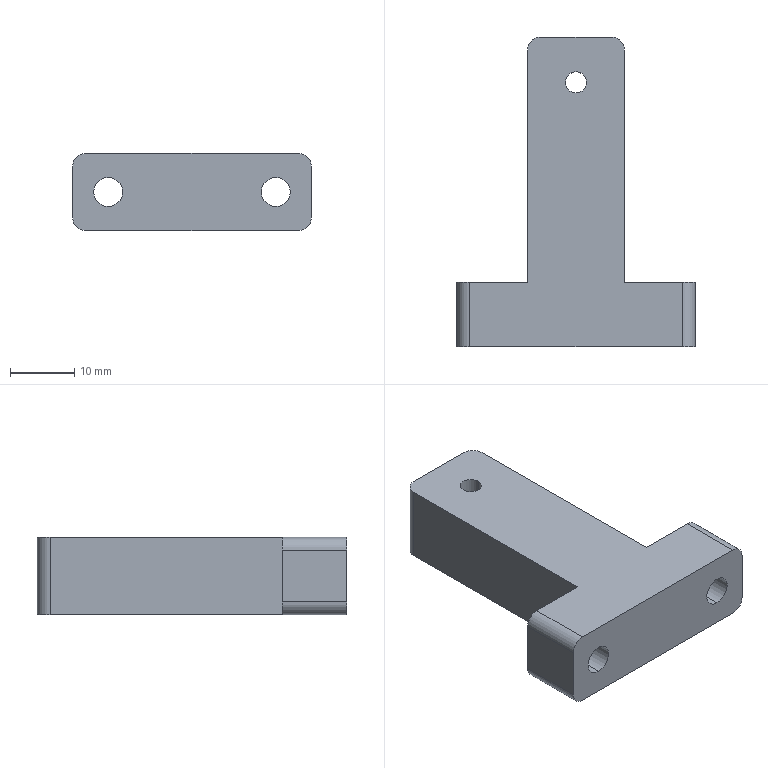Part | NX | features BREP 1 | 1 solid | 28 faces | box 37 x 48 x 12 mm | volume 10327 mm3 | cylinder 16 | plane 12 | commonest cylinder face diameters 4 x6 4.5 x4 9 x4 3.3 x2
STEP:
#1=CARTESIAN_POINT('',(7.5,46.,6.));
#2=VERTEX_POINT('',#1);
#3=CARTESIAN_POINT('',(5.5,48.,6.));
#4=VERTEX_POINT('',#3);
#5=CARTESIAN_POINT('',(5.5,46.,6.));
#6=DIRECTION('',(0.,0.,1.));
#7=DIRECTION('',(-1.,0.,0.));
#8=AXIS2_PLACEMENT_3D('',#5,#6,#7);
#9=CIRCLE('',#8,2.);
#10=EDGE_CURVE('',#2,#4,#9,.T.);
#11=ORIENTED_EDGE('',*,*,#10,.F.);
#12=CARTESIAN_POINT('',(7.5,46.,-6.));
#13=VERTEX_POINT('',#12);
#14=CARTESIAN_POINT('',(7.5,46.,6.));
#15=DIRECTION('',(0.,0.,1.));
#16=VECTOR('',#15,1000.);
#17=LINE('',#14,#16);
#18=EDGE_CURVE('',#13,#2,#17,.T.);
#19=ORIENTED_EDGE('',*,*,#18,.F.);
#20=CARTESIAN_POINT('',(5.5,48.,-6.));
#21=VERTEX_POINT('',#20);
#22=CARTESIAN_POINT('',(5.5,46.,-6.));
#23=DIRECTION('',(0.,0.,-1.));
#24=DIRECTION('',(-1.,0.,0.));
#25=AXIS2_PLACEMENT_3D('',#22,#23,#24);
#26=CIRCLE('',#25,2.);
#27=EDGE_CURVE('',#21,#13,#26,.T.);
#28=ORIENTED_EDGE('',*,*,#27,.F.);
#29=CARTESIAN_POINT('',(5.5,48.,6.));
#30=DIRECTION('',(0.,0.,-1.));
#31=VECTOR('',#30,1000.);
#32=LINE('',#29,#31);
#33=EDGE_CURVE('',#4,#21,#32,.T.);
#34=ORIENTED_EDGE('',*,*,#33,.F.);
#35=EDGE_LOOP('',(#11,#19,#28,#34));
#36=FACE_BOUND('',#35,.T.);
#37=CARTESIAN_POINT('',(5.5,46.,6.));
#38=DIRECTION('',(0.,0.,-1.));
#39=DIRECTION('',(-1.,0.,0.));
#40=AXIS2_PLACEMENT_3D('',#37,#38,#39);
#41=CYLINDRICAL_SURFACE('',#40,2.);
#42=ADVANCED_FACE('',(#36),#41,.T.);
#43=CARTESIAN_POINT('',(-5.5,48.,6.));
#44=VERTEX_POINT('',#43);
#45=CARTESIAN_POINT('',(-7.5,46.,6.));
#46=VERTEX_POINT('',#45);
#47=CARTESIAN_POINT('',(-5.5,46.,6.));
#48=DIRECTION('',(0.,0.,1.));
#49=DIRECTION('',(-1.,0.,0.));
#50=AXIS2_PLACEMENT_3D('',#47,#48,#49);
#51=CIRCLE('',#50,2.);
#52=EDGE_CURVE('',#44,#46,#51,.T.);
#53=ORIENTED_EDGE('',*,*,#52,.F.);
#54=CARTESIAN_POINT('',(-5.5,48.,-6.));
#55=VERTEX_POINT('',#54);
#56=CARTESIAN_POINT('',(-5.5,48.,6.));
#57=DIRECTION('',(0.,0.,1.));
#58=VECTOR('',#57,1000.);
#59=LINE('',#56,#58);
#60=EDGE_CURVE('',#55,#44,#59,.T.);
#61=ORIENTED_EDGE('',*,*,#60,.F.);
#62=CARTESIAN_POINT('',(-7.5,46.,-6.));
#63=VERTEX_POINT('',#62);
#64=CARTESIAN_POINT('',(-5.5,46.,-6.));
#65=DIRECTION('',(0.,0.,-1.));
#66=DIRECTION('',(-1.,0.,0.));
#67=AXIS2_PLACEMENT_3D('',#64,#65,#66);
#68=CIRCLE('',#67,2.);
#69=EDGE_CURVE('',#63,#55,#68,.T.);
#70=ORIENTED_EDGE('',*,*,#69,.F.);
#71=CARTESIAN_POINT('',(-7.5,46.,6.));
#72=DIRECTION('',(0.,0.,-1.));
#73=VECTOR('',#72,1000.);
#74=LINE('',#71,#73);
#75=EDGE_CURVE('',#46,#63,#74,.T.);
#76=ORIENTED_EDGE('',*,*,#75,.F.);
#77=EDGE_LOOP('',(#53,#61,#70,#76));
#78=FACE_BOUND('',#77,.T.);
#79=CARTESIAN_POINT('',(-5.5,46.,6.));
#80=DIRECTION('',(0.,0.,-1.));
#81=DIRECTION('',(-1.,0.,0.));
#82=AXIS2_PLACEMENT_3D('',#79,#80,#81);
#83=CYLINDRICAL_SURFACE('',#82,2.);
#84=ADVANCED_FACE('',(#78),#83,.T.);
#85=CARTESIAN_POINT('',(16.5,0.,-6.));
#86=VERTEX_POINT('',#85);
#87=CARTESIAN_POINT('',(18.5,0.,-4.));
#88=VERTEX_POINT('',#87);
#89=CARTESIAN_POINT('',(16.5,0.,-4.));
#90=DIRECTION('',(0.,-1.,0.));
#91=DIRECTION('',(0.,0.,1.));
#92=AXIS2_PLACEMENT_3D('',#89,#90,#91);
#93=CIRCLE('',#92,2.);
#94=EDGE_CURVE('',#86,#88,#93,.T.);
#95=ORIENTED_EDGE('',*,*,#94,.F.);
#96=CARTESIAN_POINT('',(16.5,10.,-6.));
#97=VERTEX_POINT('',#96);
#98=CARTESIAN_POINT('',(16.5,0.,-6.));
#99=DIRECTION('',(0.,-1.,0.));
#100=VECTOR('',#99,1000.);
#101=LINE('',#98,#100);
#102=EDGE_CURVE('',#97,#86,#101,.T.);
#103=ORIENTED_EDGE('',*,*,#102,.F.);
#104=CARTESIAN_POINT('',(18.5,10.,-4.));
#105=VERTEX_POINT('',#104);
#106=CARTESIAN_POINT('',(16.5,10.,-4.));
#107=DIRECTION('',(0.,1.,0.));
#108=DIRECTION('',(1.,0.,0.));
#109=AXIS2_PLACEMENT_3D('',#106,#107,#108);
#110=CIRCLE('',#109,2.);
#111=EDGE_CURVE('',#105,#97,#110,.T.);
#112=ORIENTED_EDGE('',*,*,#111,.F.);
#113=CARTESIAN_POINT('',(18.5,10.,-4.));
#114=DIRECTION('',(0.,1.,0.));
#115=VECTOR('',#114,1000.);
#116=LINE('',#113,#115);
#117=EDGE_CURVE('',#88,#105,#116,.T.);
#118=ORIENTED_EDGE('',*,*,#117,.F.);
#119=EDGE_LOOP('',(#95,#103,#112,#118));
#120=FACE_BOUND('',#119,.T.);
#121=CARTESIAN_POINT('',(16.5,10.,-4.));
#122=DIRECTION('',(0.,-1.,0.));
#123=DIRECTION('',(1.,0.,0.));
#124=AXIS2_PLACEMENT_3D('',#121,#122,#123);
#125=CYLINDRICAL_SURFACE('',#124,2.);
#126=ADVANCED_FACE('',(#120),#125,.T.);
#127=CARTESIAN_POINT('',(18.5,0.,4.));
#128=VERTEX_POINT('',#127);
#129=CARTESIAN_POINT('',(16.5,0.,6.));
#130=VERTEX_POINT('',#129);
#131=CARTESIAN_POINT('',(16.5,0.,4.));
#132=DIRECTION('',(0.,-1.,0.));
#133=DIRECTION('',(0.,0.,1.));
#134=AXIS2_PLACEMENT_3D('',#131,#132,#133);
#135=CIRCLE('',#134,2.);
#136=EDGE_CURVE('',#128,#130,#135,.T.);
#137=ORIENTED_EDGE('',*,*,#136,.F.);
#138=CARTESIAN_POINT('',(18.5,10.,4.));
#139=VERTEX_POINT('',#138);
#140=CARTESIAN_POINT('',(18.5,10.,4.));
#141=DIRECTION('',(0.,-1.,0.));
#142=VECTOR('',#141,1000.);
#143=LINE('',#140,#142);
#144=EDGE_CURVE('',#139,#128,#143,.T.);
#145=ORIENTED_EDGE('',*,*,#144,.F.);
#146=CARTESIAN_POINT('',(16.5,10.,6.));
#147=VERTEX_POINT('',#146);
#148=CARTESIAN_POINT('',(16.5,10.,4.));
#149=DIRECTION('',(0.,1.,0.));
#150=DIRECTION('',(1.,0.,0.));
#151=AXIS2_PLACEMENT_3D('',#148,#149,#150);
#152=CIRCLE('',#151,2.);
#153=EDGE_CURVE('',#147,#139,#152,.T.);
#154=ORIENTED_EDGE('',*,*,#153,.F.);
#155=CARTESIAN_POINT('',(16.5,0.,6.));
#156=DIRECTION('',(0.,1.,0.));
#157=VECTOR('',#156,1000.);
#158=LINE('',#155,#157);
#159=EDGE_CURVE('',#130,#147,#158,.T.);
#160=ORIENTED_EDGE('',*,*,#159,.F.);
#161=EDGE_LOOP('',(#137,#145,#154,#160));
#162=FACE_BOUND('',#161,.T.);
#163=CARTESIAN_POINT('',(16.5,0.,4.));
#164=DIRECTION('',(0.,1.,0.));
#165=DIRECTION('',(-1.,0.,0.));
#166=AXIS2_PLACEMENT_3D('',#163,#164,#165);
#167=CYLINDRICAL_SURFACE('',#166,2.);
#168=ADVANCED_FACE('',(#162),#167,.T.);
#169=CARTESIAN_POINT('',(-16.5,10.,-6.));
#170=VERTEX_POINT('',#169);
#171=CARTESIAN_POINT('',(-18.5,10.,-4.));
#172=VERTEX_POINT('',#171);
#173=CARTESIAN_POINT('',(-16.5,10.,-4.));
#174=DIRECTION('',(0.,1.,0.));
#175=DIRECTION('',(1.,0.,0.));
#176=AXIS2_PLACEMENT_3D('',#173,#174,#175);
#177=CIRCLE('',#176,2.);
#178=EDGE_CURVE('',#170,#172,#177,.T.);
#179=ORIENTED_EDGE('',*,*,#178,.F.);
#180=CARTESIAN_POINT('',(-16.5,0.,-6.));
#181=VERTEX_POINT('',#180);
#182=CARTESIAN_POINT('',(-16.5,10.,-6.));
#183=DIRECTION('',(0.,1.,0.));
#184=VECTOR('',#183,1000.);
#185=LINE('',#182,#184);
#186=EDGE_CURVE('',#181,#170,#185,.T.);
#187=ORIENTED_EDGE('',*,*,#186,.F.);
#188=CARTESIAN_POINT('',(-18.5,0.,-4.));
#189=VERTEX_POINT('',#188);
#190=CARTESIAN_POINT('',(-16.5,0.,-4.));
#191=DIRECTION('',(0.,-1.,0.));
#192=DIRECTION('',(0.,0.,1.));
#193=AXIS2_PLACEMENT_3D('',#190,#191,#192);
#194=CIRCLE('',#193,2.);
#195=EDGE_CURVE('',#189,#181,#194,.T.);
#196=ORIENTED_EDGE('',*,*,#195,.F.);
#197=CARTESIAN_POINT('',(-18.5,0.,-4.));
#198=DIRECTION('',(0.,-1.,0.));
#199=VECTOR('',#198,1000.);
#200=LINE('',#197,#199);
#201=EDGE_CURVE('',#172,#189,#200,.T.);
#202=ORIENTED_EDGE('',*,*,#201,.F.);
#203=EDGE_LOOP('',(#179,#187,#196,#202));
#204=FACE_BOUND('',#203,.T.);
#205=CARTESIAN_POINT('',(-16.5,10.,-4.));
#206=DIRECTION('',(0.,1.,0.));
#207=DIRECTION('',(-1.,0.,0.));
#208=AXIS2_PLACEMENT_3D('',#205,#206,#207);
#209=CYLINDRICAL_SURFACE('',#208,2.);
#210=ADVANCED_FACE('',(#204),#209,.T.);
#211=CARTESIAN_POINT('',(-18.5,10.,4.));
#212=VERTEX_POINT('',#211);
#213=CARTESIAN_POINT('',(-16.5,10.,6.));
#214=VERTEX_POINT('',#213);
#215=CARTESIAN_POINT('',(-16.5,10.,4.));
#216=DIRECTION('',(0.,1.,0.));
#217=DIRECTION('',(1.,0.,0.));
#218=AXIS2_PLACEMENT_3D('',#215,#216,#217);
#219=CIRCLE('',#218,2.);
#220=EDGE_CURVE('',#212,#214,#219,.T.);
#221=ORIENTED_EDGE('',*,*,#220,.F.);
#222=CARTESIAN_POINT('',(-18.5,0.,4.));
#223=VERTEX_POINT('',#222);
#224=CARTESIAN_POINT('',(-18.5,10.,4.));
#225=DIRECTION('',(0.,1.,0.));
#226=VECTOR('',#225,1000.);
#227=LINE('',#224,#226);
#228=EDGE_CURVE('',#223,#212,#227,.T.);
#229=ORIENTED_EDGE('',*,*,#228,.F.);
#230=CARTESIAN_POINT('',(-16.5,0.,6.));
#231=VERTEX_POINT('',#230);
#232=CARTESIAN_POINT('',(-16.5,0.,4.));
#233=DIRECTION('',(0.,-1.,0.));
#234=DIRECTION('',(0.,0.,1.));
#235=AXIS2_PLACEMENT_3D('',#232,#233,#234);
#236=CIRCLE('',#235,2.);
#237=EDGE_CURVE('',#231,#223,#236,.T.);
#238=ORIENTED_EDGE('',*,*,#237,.F.);
#239=CARTESIAN_POINT('',(-16.5,0.,6.));
#240=DIRECTION('',(0.,-1.,0.));
#241=VECTOR('',#240,1000.);
#242=LINE('',#239,#241);
#243=EDGE_CURVE('',#214,#231,#242,.T.);
#244=ORIENTED_EDGE('',*,*,#243,.F.);
#245=EDGE_LOOP('',(#221,#229,#238,#244));
#246=FACE_BOUND('',#245,.T.);
#247=CARTESIAN_POINT('',(-16.5,0.,4.));
#248=DIRECTION('',(0.,-1.,0.));
#249=DIRECTION('',(1.,0.,0.));
#250=AXIS2_PLACEMENT_3D('',#247,#248,#249);
#251=CYLINDRICAL_SURFACE('',#250,2.);
#252=ADVANCED_FACE('',(#246),#251,.T.);
#253=CARTESIAN_POINT('',(-1.65,41.,6.));
#254=VERTEX_POINT('',#253);
#255=CARTESIAN_POINT('',(-1.65,41.,-6.));
#256=VERTEX_POINT('',#255);
#257=CARTESIAN_POINT('',(-1.65,41.,6.));
#258=DIRECTION('',(0.,0.,1.));
#259=VECTOR('',#258,1000.);
#260=LINE('',#257,#259);
#261=EDGE_CURVE('',#254,#256,#260,.F.);
#262=ORIENTED_EDGE('',*,*,#261,.T.);
#263=CARTESIAN_POINT('',(1.65,41.,-6.));
#264=VERTEX_POINT('',#263);
#265=CARTESIAN_POINT('',(0.,41.,-6.));
#266=DIRECTION('',(0.,0.,-1.));
#267=DIRECTION('',(-1.,0.,0.));
#268=AXIS2_PLACEMENT_3D('',#265,#266,#267);
#269=CIRCLE('',#268,1.65);
#270=EDGE_CURVE('',#256,#264,#269,.T.);
#271=ORIENTED_EDGE('',*,*,#270,.T.);
#272=CARTESIAN_POINT('',(1.65,41.,6.));
#273=VERTEX_POINT('',#272);
#274=CARTESIAN_POINT('',(1.65,41.,6.));
#275=DIRECTION('',(0.,0.,1.));
#276=VECTOR('',#275,1000.);
#277=LINE('',#274,#276);
#278=EDGE_CURVE('',#273,#264,#277,.F.);
#279=ORIENTED_EDGE('',*,*,#278,.F.);
#280=CARTESIAN_POINT('',(0.,41.,6.));
#281=DIRECTION('',(0.,0.,1.));
#282=DIRECTION('',(1.,0.,0.));
#283=AXIS2_PLACEMENT_3D('',#280,#281,#282);
#284=CIRCLE('',#283,1.65);
#285=EDGE_CURVE('',#273,#254,#284,.T.);
#286=ORIENTED_EDGE('',*,*,#285,.T.);
#287=EDGE_LOOP('',(#262,#271,#279,#286));
#288=FACE_BOUND('',#287,.T.);
#289=CARTESIAN_POINT('',(0.,41.,6.));
#290=DIRECTION('',(0.,0.,1.));
#291=DIRECTION('',(1.,0.,0.));
#292=AXIS2_PLACEMENT_3D('',#289,#290,#291);
#293=CYLINDRICAL_SURFACE('',#292,1.65);
#294=ADVANCED_FACE('',(#288),#293,.F.);
#295=CARTESIAN_POINT('',(13.,10.,-4.5));
#296=VERTEX_POINT('',#295);
#297=CARTESIAN_POINT('',(13.,5.,-4.5));
#298=VERTEX_POINT('',#297);
#299=CARTESIAN_POINT('',(13.,10.,-4.5));
#300=DIRECTION('',(0.,1.,0.));
#301=VECTOR('',#300,1000.);
#302=LINE('',#299,#301);
#303=EDGE_CURVE('',#296,#298,#302,.F.);
#304=ORIENTED_EDGE('',*,*,#303,.T.);
#305=CARTESIAN_POINT('',(13.,5.,4.5));
#306=VERTEX_POINT('',#305);
#307=CARTESIAN_POINT('',(13.,5.,0.));
#308=DIRECTION('',(0.,1.,0.));
#309=DIRECTION('',(0.,0.,1.));
#310=AXIS2_PLACEMENT_3D('',#307,#308,#309);
#311=CIRCLE('',#310,4.5);
#312=EDGE_CURVE('',#306,#298,#311,.T.);
#313=ORIENTED_EDGE('',*,*,#312,.F.);
#314=CARTESIAN_POINT('',(13.,10.,4.5));
#315=VERTEX_POINT('',#314);
#316=CARTESIAN_POINT('',(13.,10.,4.5));
#317=DIRECTION('',(0.,1.,0.));
#318=VECTOR('',#317,1000.);
#319=LINE('',#316,#318);
#320=EDGE_CURVE('',#315,#306,#319,.F.);
#321=ORIENTED_EDGE('',*,*,#320,.F.);
#322=CARTESIAN_POINT('',(13.,10.,0.));
#323=DIRECTION('',(0.,1.,0.));
#324=DIRECTION('',(0.,0.,1.));
#325=AXIS2_PLACEMENT_3D('',#322,#323,#324);
#326=CIRCLE('',#325,4.5);
#327=EDGE_CURVE('',#315,#296,#326,.T.);
#328=ORIENTED_EDGE('',*,*,#327,.T.);
#329=EDGE_LOOP('',(#304,#313,#321,#328));
#330=FACE_BOUND('',#329,.T.);
#331=CARTESIAN_POINT('',(13.,10.,0.));
#332=DIRECTION('',(0.,1.,0.));
#333=DIRECTION('',(0.,0.,1.));
#334=AXIS2_PLACEMENT_3D('',#331,#332,#333);
#335=CYLINDRICAL_SURFACE('',#334,4.5);
#336=ADVANCED_FACE('',(#330),#335,.F.);
#337=ORIENTED_EDGE('',*,*,#312,.T.);
#338=CARTESIAN_POINT('',(13.,5.,0.));
#339=DIRECTION('',(0.,1.,0.));
#340=DIRECTION('',(0.,0.,1.));
#341=AXIS2_PLACEMENT_3D('',#338,#339,#340);
#342=CIRCLE('',#341,4.5);
#343=EDGE_CURVE('',#298,#306,#342,.T.);
#344=ORIENTED_EDGE('',*,*,#343,.T.);
#345=EDGE_LOOP('',(#337,#344));
#346=FACE_BOUND('',#345,.T.);
#347=CARTESIAN_POINT('',(13.,5.,2.25));
#348=VERTEX_POINT('',#347);
#349=CARTESIAN_POINT('',(13.,5.,-2.25));
#350=VERTEX_POINT('',#349);
#351=CARTESIAN_POINT('',(13.,5.,0.));
#352=DIRECTION('',(0.,1.,0.));
#353=DIRECTION('',(0.,0.,1.));
#354=AXIS2_PLACEMENT_3D('',#351,#352,#353);
#355=CIRCLE('',#354,2.25);
#356=EDGE_CURVE('',#348,#350,#355,.T.);
#357=ORIENTED_EDGE('',*,*,#356,.F.);
#358=CARTESIAN_POINT('',(13.,5.,0.));
#359=DIRECTION('',(0.,1.,0.));
#360=DIRECTION('',(0.,0.,1.));
#361=AXIS2_PLACEMENT_3D('',#358,#359,#360);
#362=CIRCLE('',#361,2.25);
#363=EDGE_CURVE('',#350,#348,#362,.T.);
#364=ORIENTED_EDGE('',*,*,#363,.F.);
#365=EDGE_LOOP('',(#357,#364));
#366=FACE_BOUND('',#365,.T.);
#367=CARTESIAN_POINT('',(15.25,5.,0.));
#368=DIRECTION('',(0.,-1.,0.));
#369=DIRECTION('',(0.,0.,-1.));
#370=AXIS2_PLACEMENT_3D('',#367,#368,#369);
#371=PLANE('',#370);
#372=ADVANCED_FACE('',(#346,#366),#371,.F.);
#373=CARTESIAN_POINT('',(13.,0.,-2.25));
#374=VERTEX_POINT('',#373);
#375=CARTESIAN_POINT('',(13.,10.,-2.25));
#376=DIRECTION('',(0.,1.,0.));
#377=VECTOR('',#376,1000.);
#378=LINE('',#375,#377);
#379=EDGE_CURVE('',#350,#374,#378,.F.);
#380=ORIENTED_EDGE('',*,*,#379,.T.);
#381=CARTESIAN_POINT('',(13.,0.,2.25));
#382=VERTEX_POINT('',#381);
#383=CARTESIAN_POINT('',(13.,0.,0.));
#384=DIRECTION('',(0.,1.,0.));
#385=DIRECTION('',(0.,0.,1.));
#386=AXIS2_PLACEMENT_3D('',#383,#384,#385);
#387=CIRCLE('',#386,2.25);
#388=EDGE_CURVE('',#382,#374,#387,.T.);
#389=ORIENTED_EDGE('',*,*,#388,.F.);
#390=CARTESIAN_POINT('',(13.,10.,2.25));
#391=DIRECTION('',(0.,1.,0.));
#392=VECTOR('',#391,1000.);
#393=LINE('',#390,#392);
#394=EDGE_CURVE('',#348,#382,#393,.F.);
#395=ORIENTED_EDGE('',*,*,#394,.F.);
#396=ORIENTED_EDGE('',*,*,#356,.T.);
#397=EDGE_LOOP('',(#380,#389,#395,#396));
#398=FACE_BOUND('',#397,.T.);
#399=CARTESIAN_POINT('',(13.,10.,0.));
#400=DIRECTION('',(0.,1.,0.));
#401=DIRECTION('',(0.,0.,1.));
#402=AXIS2_PLACEMENT_3D('',#399,#400,#401);
#403=CYLINDRICAL_SURFACE('',#402,2.25);
#404=ADVANCED_FACE('',(#398),#403,.F.);
#405=CARTESIAN_POINT('',(-13.,10.,-4.5));
#406=VERTEX_POINT('',#405);
#407=CARTESIAN_POINT('',(-13.,5.,-4.5));
#408=VERTEX_POINT('',#407);
#409=CARTESIAN_POINT('',(-13.,10.,-4.5));
#410=DIRECTION('',(0.,1.,0.));
#411=VECTOR('',#410,1000.);
#412=LINE('',#409,#411);
#413=EDGE_CURVE('',#406,#408,#412,.F.);
#414=ORIENTED_EDGE('',*,*,#413,.T.);
#415=CARTESIAN_POINT('',(-13.,5.,4.5));
#416=VERTEX_POINT('',#415);
#417=CARTESIAN_POINT('',(-13.,5.,0.));
#418=DIRECTION('',(0.,1.,0.));
#419=DIRECTION('',(0.,0.,1.));
#420=AXIS2_PLACEMENT_3D('',#417,#418,#419);
#421=CIRCLE('',#420,4.5);
#422=EDGE_CURVE('',#416,#408,#421,.T.);
#423=ORIENTED_EDGE('',*,*,#422,.F.);
#424=CARTESIAN_POINT('',(-13.,10.,4.5));
#425=VERTEX_POINT('',#424);
#426=CARTESIAN_POINT('',(-13.,10.,4.5));
#427=DIRECTION('',(0.,1.,0.));
#428=VECTOR('',#427,1000.);
#429=LINE('',#426,#428);
#430=EDGE_CURVE('',#425,#416,#429,.F.);
#431=ORIENTED_EDGE('',*,*,#430,.F.);
#432=CARTESIAN_POINT('',(-13.,10.,0.));
#433=DIRECTION('',(0.,1.,0.));
#434=DIRECTION('',(0.,0.,1.));
#435=AXIS2_PLACEMENT_3D('',#432,#433,#434);
#436=CIRCLE('',#435,4.5);
#437=EDGE_CURVE('',#425,#406,#436,.T.);
#438=ORIENTED_EDGE('',*,*,#437,.T.);
#439=EDGE_LOOP('',(#414,#423,#431,#438));
#440=FACE_BOUND('',#439,.T.);
#441=CARTESIAN_POINT('',(-13.,10.,0.));
#442=DIRECTION('',(0.,1.,0.));
#443=DIRECTION('',(0.,0.,1.));
#444=AXIS2_PLACEMENT_3D('',#441,#442,#443);
#445=CYLINDRICAL_SURFACE('',#444,4.5);
#446=ADVANCED_FACE('',(#440),#445,.F.);
#447=ORIENTED_EDGE('',*,*,#422,.T.);
#448=CARTESIAN_POINT('',(-13.,5.,0.));
#449=DIRECTION('',(0.,1.,0.));
#450=DIRECTION('',(0.,0.,1.));
#451=AXIS2_PLACEMENT_3D('',#448,#449,#450);
#452=CIRCLE('',#451,4.5);
#453=EDGE_CURVE('',#408,#416,#452,.T.);
#454=ORIENTED_EDGE('',*,*,#453,.T.);
#455=EDGE_LOOP('',(#447,#454));
#456=FACE_BOUND('',#455,.T.);
#457=CARTESIAN_POINT('',(-13.,5.,2.25));
#458=VERTEX_POINT('',#457);
#459=CARTESIAN_POINT('',(-13.,5.,-2.25));
#460=VERTEX_POINT('',#459);
#461=CARTESIAN_POINT('',(-13.,5.,0.));
#462=DIRECTION('',(0.,1.,0.));
#463=DIRECTION('',(0.,0.,1.));
#464=AXIS2_PLACEMENT_3D('',#461,#462,#463);
#465=CIRCLE('',#464,2.25);
#466=EDGE_CURVE('',#458,#460,#465,.T.);
#467=ORIENTED_EDGE('',*,*,#466,.F.);
#468=CARTESIAN_POINT('',(-13.,5.,0.));
#469=DIRECTION('',(0.,1.,0.));
#470=DIRECTION('',(0.,0.,1.));
#471=AXIS2_PLACEMENT_3D('',#468,#469,#470);
#472=CIRCLE('',#471,2.25);
#473=EDGE_CURVE('',#460,#458,#472,.T.);
#474=ORIENTED_EDGE('',*,*,#473,.F.);
#475=EDGE_LOOP('',(#467,#474));
#476=FACE_BOUND('',#475,.T.);
#477=CARTESIAN_POINT('',(-10.75,5.,0.));
#478=DIRECTION('',(0.,-1.,0.));
#479=DIRECTION('',(0.,0.,-1.));
#480=AXIS2_PLACEMENT_3D('',#477,#478,#479);
#481=PLANE('',#480);
#482=ADVANCED_FACE('',(#456,#476),#481,.F.);
#483=CARTESIAN_POINT('',(-13.,0.,-2.25));
#484=VERTEX_POINT('',#483);
#485=CARTESIAN_POINT('',(-13.,10.,-2.25));
#486=DIRECTION('',(0.,1.,0.));
#487=VECTOR('',#486,1000.);
#488=LINE('',#485,#487);
#489=EDGE_CURVE('',#460,#484,#488,.F.);
#490=ORIENTED_EDGE('',*,*,#489,.T.);
#491=CARTESIAN_POINT('',(-13.,0.,2.25));
#492=VERTEX_POINT('',#491);
#493=CARTESIAN_POINT('',(-13.,0.,0.));
#494=DIRECTION('',(0.,1.,0.));
#495=DIRECTION('',(0.,0.,1.));
#496=AXIS2_PLACEMENT_3D('',#493,#494,#495);
#497=CIRCLE('',#496,2.25);
#498=EDGE_CURVE('',#492,#484,#497,.T.);
#499=ORIENTED_EDGE('',*,*,#498,.F.);
#500=CARTESIAN_POINT('',(-13.,10.,2.25));
#501=DIRECTION('',(0.,1.,0.));
#502=VECTOR('',#501,1000.);
#503=LINE('',#500,#502);
#504=EDGE_CURVE('',#458,#492,#503,.F.);
#505=ORIENTED_EDGE('',*,*,#504,.F.);
#506=ORIENTED_EDGE('',*,*,#466,.T.);
#507=EDGE_LOOP('',(#490,#499,#505,#506));
#508=FACE_BOUND('',#507,.T.);
#509=CARTESIAN_POINT('',(-13.,10.,0.));
#510=DIRECTION('',(0.,1.,0.));
#511=DIRECTION('',(0.,0.,1.));
#512=AXIS2_PLACEMENT_3D('',#509,#510,#511);
#513=CYLINDRICAL_SURFACE('',#512,2.25);
#514=ADVANCED_FACE('',(#508),#513,.F.);
#515=CARTESIAN_POINT('',(-18.5,0.,-6.));
#516=DIRECTION('',(1.,0.,0.));
#517=VECTOR('',#516,1000.);
#518=LINE('',#515,#517);
#519=EDGE_CURVE('',#181,#86,#518,.T.);
#520=ORIENTED_EDGE('',*,*,#519,.F.);
#521=ORIENTED_EDGE('',*,*,#186,.T.);
#522=CARTESIAN_POINT('',(-7.5,10.,-6.));
#523=VERTEX_POINT('',#522);
#524=CARTESIAN_POINT('',(-7.5,10.,-6.));
#525=DIRECTION('',(-1.,0.,0.));
#526=VECTOR('',#525,1000.);
#527=LINE('',#524,#526);
#528=EDGE_CURVE('',#523,#170,#527,.T.);
#529=ORIENTED_EDGE('',*,*,#528,.F.);
#530=CARTESIAN_POINT('',(-7.5,48.,-6.));
#531=DIRECTION('',(0.,-1.,0.));
#532=VECTOR('',#531,1000.);
#533=LINE('',#530,#532);
#534=EDGE_CURVE('',#63,#523,#533,.T.);
#535=ORIENTED_EDGE('',*,*,#534,.F.);
#536=ORIENTED_EDGE('',*,*,#69,.T.);
#537=CARTESIAN_POINT('',(7.5,48.,-6.));
#538=DIRECTION('',(-1.,0.,0.));
#539=VECTOR('',#538,1000.);
#540=LINE('',#537,#539);
#541=EDGE_CURVE('',#21,#55,#540,.T.);
#542=ORIENTED_EDGE('',*,*,#541,.F.);
#543=ORIENTED_EDGE('',*,*,#27,.T.);
#544=CARTESIAN_POINT('',(7.5,10.,-6.));
#545=VERTEX_POINT('',#544);
#546=CARTESIAN_POINT('',(7.5,48.,-6.));
#547=DIRECTION('',(0.,1.,0.));
#548=VECTOR('',#547,1000.);
#549=LINE('',#546,#548);
#550=EDGE_CURVE('',#545,#13,#549,.T.);
#551=ORIENTED_EDGE('',*,*,#550,.F.);
#552=CARTESIAN_POINT('',(7.5,10.,-6.));
#553=DIRECTION('',(-1.,0.,0.));
#554=VECTOR('',#553,1000.);
#555=LINE('',#552,#554);
#556=EDGE_CURVE('',#97,#545,#555,.T.);
#557=ORIENTED_EDGE('',*,*,#556,.F.);
#558=ORIENTED_EDGE('',*,*,#102,.T.);
#559=EDGE_LOOP('',(#520,#521,#529,#535,#536,#542,#543,#551,#557,#558));
#560=FACE_BOUND('',#559,.T.);
#561=CARTESIAN_POINT('',(0.,41.,-6.));
#562=DIRECTION('',(0.,0.,-1.));
#563=DIRECTION('',(-1.,0.,0.));
#564=AXIS2_PLACEMENT_3D('',#561,#562,#563);
#565=CIRCLE('',#564,1.65);
#566=EDGE_CURVE('',#264,#256,#565,.T.);
#567=ORIENTED_EDGE('',*,*,#566,.F.);
#568=ORIENTED_EDGE('',*,*,#270,.F.);
#569=EDGE_LOOP('',(#567,#568));
#570=FACE_BOUND('',#569,.T.);
#571=CARTESIAN_POINT('',(0.,0.,-6.));
#572=DIRECTION('',(0.,0.,-1.));
#573=DIRECTION('',(-1.,0.,0.));
#574=AXIS2_PLACEMENT_3D('',#571,#572,#573);
#575=PLANE('',#574);
#576=ADVANCED_FACE('',(#560,#570),#575,.T.);
#577=ORIENTED_EDGE('',*,*,#541,.T.);
#578=ORIENTED_EDGE('',*,*,#60,.T.);
#579=CARTESIAN_POINT('',(7.5,48.,6.));
#580=DIRECTION('',(-1.,0.,0.));
#581=VECTOR('',#580,1000.);
#582=LINE('',#579,#581);
#583=EDGE_CURVE('',#4,#44,#582,.T.);
#584=ORIENTED_EDGE('',*,*,#583,.F.);
#585=ORIENTED_EDGE('',*,*,#33,.T.);
#586=EDGE_LOOP('',(#577,#578,#584,#585));
#587=FACE_BOUND('',#586,.T.);
#588=CARTESIAN_POINT('',(7.5,48.,6.));
#589=DIRECTION('',(0.,-1.,0.));
#590=DIRECTION('',(0.,0.,-1.));
#591=AXIS2_PLACEMENT_3D('',#588,#589,#590);
#592=PLANE('',#591);
#593=ADVANCED_FACE('',(#587),#592,.F.);
#594=ORIENTED_EDGE('',*,*,#550,.T.);
#595=ORIENTED_EDGE('',*,*,#18,.T.);
#596=CARTESIAN_POINT('',(7.5,10.,6.));
#597=VERTEX_POINT('',#596);
#598=CARTESIAN_POINT('',(7.5,48.,6.));
#599=DIRECTION('',(0.,1.,0.));
#600=VECTOR('',#599,1000.);
#601=LINE('',#598,#600);
#602=EDGE_CURVE('',#597,#2,#601,.T.);
#603=ORIENTED_EDGE('',*,*,#602,.F.);
#604=CARTESIAN_POINT('',(7.5,10.,6.));
#605=DIRECTION('',(0.,0.,-1.));
#606=VECTOR('',#605,1000.);
#607=LINE('',#604,#606);
#608=EDGE_CURVE('',#597,#545,#607,.T.);
#609=ORIENTED_EDGE('',*,*,#608,.T.);
#610=EDGE_LOOP('',(#594,#595,#603,#609));
#611=FACE_BOUND('',#610,.T.);
#612=CARTESIAN_POINT('',(7.5,48.,6.));
#613=DIRECTION('',(-1.,0.,0.));
#614=DIRECTION('',(0.,-1.,0.));
#615=AXIS2_PLACEMENT_3D('',#612,#613,#614);
#616=PLANE('',#615);
#617=ADVANCED_FACE('',(#611),#616,.F.);
#618=CARTESIAN_POINT('',(18.5,10.,6.));
#619=DIRECTION('',(0.,0.,-1.));
#620=VECTOR('',#619,1000.);
#621=LINE('',#618,#620);
#622=EDGE_CURVE('',#139,#105,#621,.T.);
#623=ORIENTED_EDGE('',*,*,#622,.F.);
#624=ORIENTED_EDGE('',*,*,#144,.T.);
#625=CARTESIAN_POINT('',(18.5,0.,6.));
#626=DIRECTION('',(0.,0.,-1.));
#627=VECTOR('',#626,1000.);
#628=LINE('',#625,#627);
#629=EDGE_CURVE('',#128,#88,#628,.T.);
#630=ORIENTED_EDGE('',*,*,#629,.T.);
#631=ORIENTED_EDGE('',*,*,#117,.T.);
#632=EDGE_LOOP('',(#623,#624,#630,#631));
#633=FACE_BOUND('',#632,.T.);
#634=CARTESIAN_POINT('',(18.5,10.,6.));
#635=DIRECTION('',(-1.,0.,0.));
#636=DIRECTION('',(0.,-1.,0.));
#637=AXIS2_PLACEMENT_3D('',#634,#635,#636);
#638=PLANE('',#637);
#639=ADVANCED_FACE('',(#633),#638,.F.);
#640=CARTESIAN_POINT('',(-18.5,0.,6.));
#641=DIRECTION('',(1.,0.,0.));
#642=VECTOR('',#641,1000.);
#643=LINE('',#640,#642);
#644=EDGE_CURVE('',#231,#130,#643,.T.);
#645=ORIENTED_EDGE('',*,*,#644,.F.);
#646=ORIENTED_EDGE('',*,*,#237,.T.);
#647=CARTESIAN_POINT('',(-18.5,0.,6.));
#648=DIRECTION('',(0.,0.,-1.));
#649=VECTOR('',#648,1000.);
#650=LINE('',#647,#649);
#651=EDGE_CURVE('',#223,#189,#650,.T.);
#652=ORIENTED_EDGE('',*,*,#651,.T.);
#653=ORIENTED_EDGE('',*,*,#195,.T.);
#654=ORIENTED_EDGE('',*,*,#519,.T.);
#655=ORIENTED_EDGE('',*,*,#94,.T.);
#656=ORIENTED_EDGE('',*,*,#629,.F.);
#657=ORIENTED_EDGE('',*,*,#136,.T.);
#658=EDGE_LOOP('',(#645,#646,#652,#653,#654,#655,#656,#657));
#659=FACE_BOUND('',#658,.T.);
#660=ORIENTED_EDGE('',*,*,#498,.T.);
#661=CARTESIAN_POINT('',(-13.,0.,0.));
#662=DIRECTION('',(0.,1.,0.));
#663=DIRECTION('',(0.,0.,1.));
#664=AXIS2_PLACEMENT_3D('',#661,#662,#663);
#665=CIRCLE('',#664,2.25);
#666=EDGE_CURVE('',#484,#492,#665,.T.);
#667=ORIENTED_EDGE('',*,*,#666,.T.);
#668=EDGE_LOOP('',(#660,#667));
#669=FACE_BOUND('',#668,.T.);
#670=ORIENTED_EDGE('',*,*,#388,.T.);
#671=CARTESIAN_POINT('',(13.,0.,0.));
#672=DIRECTION('',(0.,1.,0.));
#673=DIRECTION('',(0.,0.,1.));
#674=AXIS2_PLACEMENT_3D('',#671,#672,#673);
#675=CIRCLE('',#674,2.25);
#676=EDGE_CURVE('',#374,#382,#675,.T.);
#677=ORIENTED_EDGE('',*,*,#676,.T.);
#678=EDGE_LOOP('',(#670,#677));
#679=FACE_BOUND('',#678,.T.);
#680=CARTESIAN_POINT('',(-18.5,0.,6.));
#681=DIRECTION('',(0.,1.,0.));
#682=DIRECTION('',(0.,0.,1.));
#683=AXIS2_PLACEMENT_3D('',#680,#681,#682);
#684=PLANE('',#683);
#685=ADVANCED_FACE('',(#659,#669,#679),#684,.F.);
#686=ORIENTED_EDGE('',*,*,#651,.F.);
#687=ORIENTED_EDGE('',*,*,#228,.T.);
#688=CARTESIAN_POINT('',(-18.5,10.,6.));
#689=DIRECTION('',(0.,0.,-1.));
#690=VECTOR('',#689,1000.);
#691=LINE('',#688,#690);
#692=EDGE_CURVE('',#212,#172,#691,.T.);
#693=ORIENTED_EDGE('',*,*,#692,.T.);
#694=ORIENTED_EDGE('',*,*,#201,.T.);
#695=EDGE_LOOP('',(#686,#687,#693,#694));
#696=FACE_BOUND('',#695,.T.);
#697=CARTESIAN_POINT('',(-18.5,10.,6.));
#698=DIRECTION('',(1.,0.,0.));
#699=DIRECTION('',(0.,1.,0.));
#700=AXIS2_PLACEMENT_3D('',#697,#698,#699);
#701=PLANE('',#700);
#702=ADVANCED_FACE('',(#696),#701,.F.);
#703=ORIENTED_EDGE('',*,*,#692,.F.);
#704=ORIENTED_EDGE('',*,*,#220,.T.);
#705=CARTESIAN_POINT('',(-7.5,10.,6.));
#706=VERTEX_POINT('',#705);
#707=CARTESIAN_POINT('',(-7.5,10.,6.));
#708=DIRECTION('',(-1.,0.,0.));
#709=VECTOR('',#708,1000.);
#710=LINE('',#707,#709);
#711=EDGE_CURVE('',#706,#214,#710,.T.);
#712=ORIENTED_EDGE('',*,*,#711,.F.);
#713=CARTESIAN_POINT('',(-7.5,10.,6.));
#714=DIRECTION('',(0.,0.,-1.));
#715=VECTOR('',#714,1000.);
#716=LINE('',#713,#715);
#717=EDGE_CURVE('',#706,#523,#716,.T.);
#718=ORIENTED_EDGE('',*,*,#717,.T.);
#719=ORIENTED_EDGE('',*,*,#528,.T.);
#720=ORIENTED_EDGE('',*,*,#178,.T.);
#721=EDGE_LOOP('',(#703,#704,#712,#718,#719,#720));
#722=FACE_BOUND('',#721,.T.);
#723=ORIENTED_EDGE('',*,*,#437,.F.);
#724=CARTESIAN_POINT('',(-13.,10.,0.));
#725=DIRECTION('',(0.,1.,0.));
#726=DIRECTION('',(0.,0.,1.));
#727=AXIS2_PLACEMENT_3D('',#724,#725,#726);
#728=CIRCLE('',#727,4.5);
#729=EDGE_CURVE('',#406,#425,#728,.T.);
#730=ORIENTED_EDGE('',*,*,#729,.F.);
#731=EDGE_LOOP('',(#723,#730));
#732=FACE_BOUND('',#731,.T.);
#733=CARTESIAN_POINT('',(-7.5,10.,6.));
#734=DIRECTION('',(0.,-1.,0.));
#735=DIRECTION('',(1.,0.,0.));
#736=AXIS2_PLACEMENT_3D('',#733,#734,#735);
#737=PLANE('',#736);
#738=ADVANCED_FACE('',(#722,#732),#737,.F.);
#739=CARTESIAN_POINT('',(-7.5,48.,6.));
#740=DIRECTION('',(0.,-1.,0.));
#741=VECTOR('',#740,1000.);
#742=LINE('',#739,#741);
#743=EDGE_CURVE('',#46,#706,#742,.T.);
#744=ORIENTED_EDGE('',*,*,#743,.F.);
#745=ORIENTED_EDGE('',*,*,#75,.T.);
#746=ORIENTED_EDGE('',*,*,#534,.T.);
#747=ORIENTED_EDGE('',*,*,#717,.F.);
#748=EDGE_LOOP('',(#744,#745,#746,#747));
#749=FACE_BOUND('',#748,.T.);
#750=CARTESIAN_POINT('',(-7.5,48.,6.));
#751=DIRECTION('',(1.,0.,0.));
#752=DIRECTION('',(0.,1.,0.));
#753=AXIS2_PLACEMENT_3D('',#750,#751,#752);
#754=PLANE('',#753);
#755=ADVANCED_FACE('',(#749),#754,.F.);
#756=ORIENTED_EDGE('',*,*,#327,.F.);
#757=CARTESIAN_POINT('',(13.,10.,0.));
#758=DIRECTION('',(0.,1.,0.));
#759=DIRECTION('',(0.,0.,1.));
#760=AXIS2_PLACEMENT_3D('',#757,#758,#759);
#761=CIRCLE('',#760,4.5);
#762=EDGE_CURVE('',#296,#315,#761,.T.);
#763=ORIENTED_EDGE('',*,*,#762,.F.);
#764=EDGE_LOOP('',(#756,#763));
#765=FACE_BOUND('',#764,.T.);
#766=CARTESIAN_POINT('',(7.5,10.,6.));
#767=DIRECTION('',(-1.,0.,0.));
#768=VECTOR('',#767,1000.);
#769=LINE('',#766,#768);
#770=EDGE_CURVE('',#147,#597,#769,.T.);
#771=ORIENTED_EDGE('',*,*,#770,.F.);
#772=ORIENTED_EDGE('',*,*,#153,.T.);
#773=ORIENTED_EDGE('',*,*,#622,.T.);
#774=ORIENTED_EDGE('',*,*,#111,.T.);
#775=ORIENTED_EDGE('',*,*,#556,.T.);
#776=ORIENTED_EDGE('',*,*,#608,.F.);
#777=EDGE_LOOP('',(#771,#772,#773,#774,#775,#776));
#778=FACE_BOUND('',#777,.T.);
#779=CARTESIAN_POINT('',(7.5,10.,6.));
#780=DIRECTION('',(0.,-1.,0.));
#781=DIRECTION('',(1.,0.,0.));
#782=AXIS2_PLACEMENT_3D('',#779,#780,#781);
#783=PLANE('',#782);
#784=ADVANCED_FACE('',(#765,#778),#783,.F.);
#785=ORIENTED_EDGE('',*,*,#285,.F.);
#786=CARTESIAN_POINT('',(0.,41.,6.));
#787=DIRECTION('',(0.,0.,1.));
#788=DIRECTION('',(1.,0.,0.));
#789=AXIS2_PLACEMENT_3D('',#786,#787,#788);
#790=CIRCLE('',#789,1.65);
#791=EDGE_CURVE('',#254,#273,#790,.T.);
#792=ORIENTED_EDGE('',*,*,#791,.F.);
#793=EDGE_LOOP('',(#785,#792));
#794=FACE_BOUND('',#793,.T.);
#795=ORIENTED_EDGE('',*,*,#711,.T.);
#796=ORIENTED_EDGE('',*,*,#243,.T.);
#797=ORIENTED_EDGE('',*,*,#644,.T.);
#798=ORIENTED_EDGE('',*,*,#159,.T.);
#799=ORIENTED_EDGE('',*,*,#770,.T.);
#800=ORIENTED_EDGE('',*,*,#602,.T.);
#801=ORIENTED_EDGE('',*,*,#10,.T.);
#802=ORIENTED_EDGE('',*,*,#583,.T.);
#803=ORIENTED_EDGE('',*,*,#52,.T.);
#804=ORIENTED_EDGE('',*,*,#743,.T.);
#805=EDGE_LOOP('',(#795,#796,#797,#798,#799,#800,#801,#802,#803,#804));
#806=FACE_BOUND('',#805,.T.);
#807=CARTESIAN_POINT('',(0.,0.,6.));
#808=DIRECTION('',(0.,0.,-1.));
#809=DIRECTION('',(-1.,0.,0.));
#810=AXIS2_PLACEMENT_3D('',#807,#808,#809);
#811=PLANE('',#810);
#812=ADVANCED_FACE('',(#794,#806),#811,.F.);
#813=ORIENTED_EDGE('',*,*,#666,.F.);
#814=ORIENTED_EDGE('',*,*,#489,.F.);
#815=ORIENTED_EDGE('',*,*,#473,.T.);
#816=ORIENTED_EDGE('',*,*,#504,.T.);
#817=EDGE_LOOP('',(#813,#814,#815,#816));
#818=FACE_BOUND('',#817,.T.);
#819=CARTESIAN_POINT('',(-13.,10.,0.));
#820=DIRECTION('',(0.,1.,0.));
#821=DIRECTION('',(0.,0.,1.));
#822=AXIS2_PLACEMENT_3D('',#819,#820,#821);
#823=CYLINDRICAL_SURFACE('',#822,2.25);
#824=ADVANCED_FACE('',(#818),#823,.F.);
#825=ORIENTED_EDGE('',*,*,#453,.F.);
#826=ORIENTED_EDGE('',*,*,#413,.F.);
#827=ORIENTED_EDGE('',*,*,#729,.T.);
#828=ORIENTED_EDGE('',*,*,#430,.T.);
#829=EDGE_LOOP('',(#825,#826,#827,#828));
#830=FACE_BOUND('',#829,.T.);
#831=CARTESIAN_POINT('',(-13.,10.,0.));
#832=DIRECTION('',(0.,1.,0.));
#833=DIRECTION('',(0.,0.,1.));
#834=AXIS2_PLACEMENT_3D('',#831,#832,#833);
#835=CYLINDRICAL_SURFACE('',#834,4.5);
#836=ADVANCED_FACE('',(#830),#835,.F.);
#837=ORIENTED_EDGE('',*,*,#676,.F.);
#838=ORIENTED_EDGE('',*,*,#379,.F.);
#839=ORIENTED_EDGE('',*,*,#363,.T.);
#840=ORIENTED_EDGE('',*,*,#394,.T.);
#841=EDGE_LOOP('',(#837,#838,#839,#840));
#842=FACE_BOUND('',#841,.T.);
#843=CARTESIAN_POINT('',(13.,10.,0.));
#844=DIRECTION('',(0.,1.,0.));
#845=DIRECTION('',(0.,0.,1.));
#846=AXIS2_PLACEMENT_3D('',#843,#844,#845);
#847=CYLINDRICAL_SURFACE('',#846,2.25);
#848=ADVANCED_FACE('',(#842),#847,.F.);
#849=ORIENTED_EDGE('',*,*,#343,.F.);
#850=ORIENTED_EDGE('',*,*,#303,.F.);
#851=ORIENTED_EDGE('',*,*,#762,.T.);
#852=ORIENTED_EDGE('',*,*,#320,.T.);
#853=EDGE_LOOP('',(#849,#850,#851,#852));
#854=FACE_BOUND('',#853,.T.);
#855=CARTESIAN_POINT('',(13.,10.,0.));
#856=DIRECTION('',(0.,1.,0.));
#857=DIRECTION('',(0.,0.,1.));
#858=AXIS2_PLACEMENT_3D('',#855,#856,#857);
#859=CYLINDRICAL_SURFACE('',#858,4.5);
#860=ADVANCED_FACE('',(#854),#859,.F.);
#861=ORIENTED_EDGE('',*,*,#566,.T.);
#862=ORIENTED_EDGE('',*,*,#261,.F.);
#863=ORIENTED_EDGE('',*,*,#791,.T.);
#864=ORIENTED_EDGE('',*,*,#278,.T.);
#865=EDGE_LOOP('',(#861,#862,#863,#864));
#866=FACE_BOUND('',#865,.T.);
#867=CARTESIAN_POINT('',(0.,41.,6.));
#868=DIRECTION('',(0.,0.,1.));
#869=DIRECTION('',(1.,0.,0.));
#870=AXIS2_PLACEMENT_3D('',#867,#868,#869);
#871=CYLINDRICAL_SURFACE('',#870,1.65);
#872=ADVANCED_FACE('',(#866),#871,.F.);
#873=CLOSED_SHELL('',(#42,#84,#126,#168,#210,#252,#294,#336,#372,#404,#446,#482,#514,#576,#593,#617,#639,#685,#702,#738,#755,#784,#812,#824,#836,#848,#860,#872));
#874=MANIFOLD_SOLID_BREP('',#873);
#875=(LENGTH_UNIT()NAMED_UNIT(*)SI_UNIT(.MILLI.,.METRE.));
#876=UNCERTAINTY_MEASURE_WITH_UNIT(LENGTH_MEASURE(0.00001),#875,'','');
#877=(NAMED_UNIT(*)PLANE_ANGLE_UNIT()SI_UNIT($,.RADIAN.));
#878=(NAMED_UNIT(*)SI_UNIT($,.STERADIAN.)SOLID_ANGLE_UNIT());
#879=(GEOMETRIC_REPRESENTATION_CONTEXT(3)GLOBAL_UNCERTAINTY_ASSIGNED_CONTEXT((#876))GLOBAL_UNIT_ASSIGNED_CONTEXT((#875,#877,#878))REPRESENTATION_CONTEXT('',''));
#880=ADVANCED_BREP_SHAPE_REPRESENTATION('',(#874),#879);